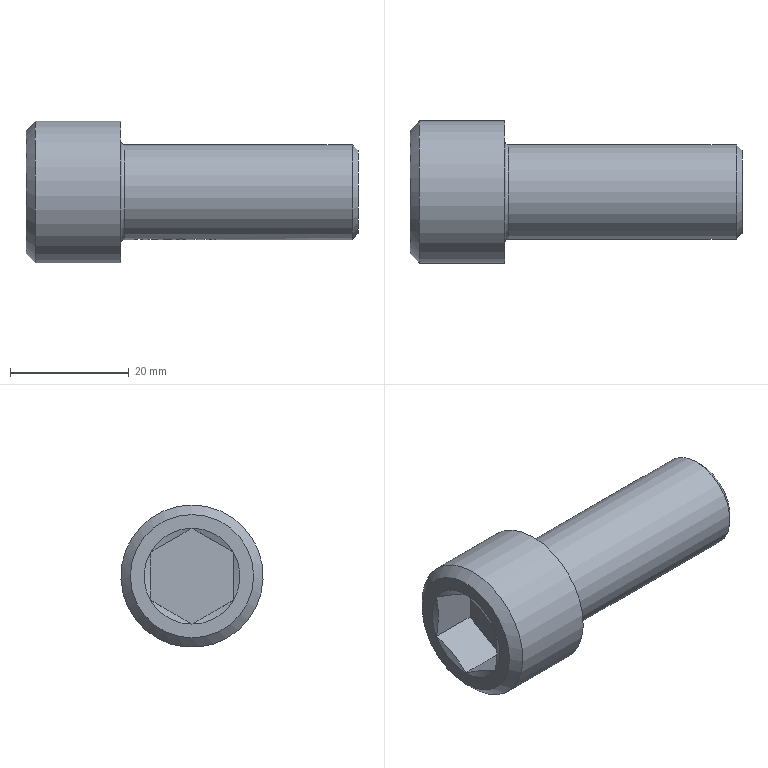Part | STEP file | solid 36 | 1 solid | 112 faces | box 56 x 24 x 24 mm | volume 13802 mm3 | plane 68 | other 27 | cylinder 8 | sphere 6 | cone 2 | torus 1 | commonest cylinder face diameters 16 x7 24 x1